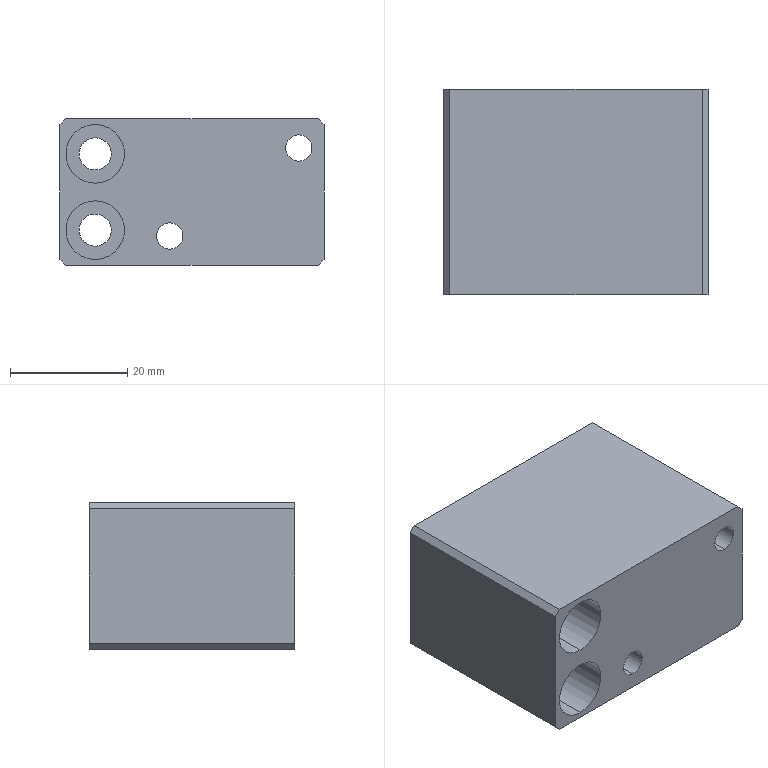Part | STEP file | PN_0049 | 1 solid | 30 faces | box 45 x 35 x 25 mm | volume 32071 mm3 | cylinder 16 | plane 14 | commonest cylinder face diameters 4.5 x4 5.5 x4 8 x4 10 x4